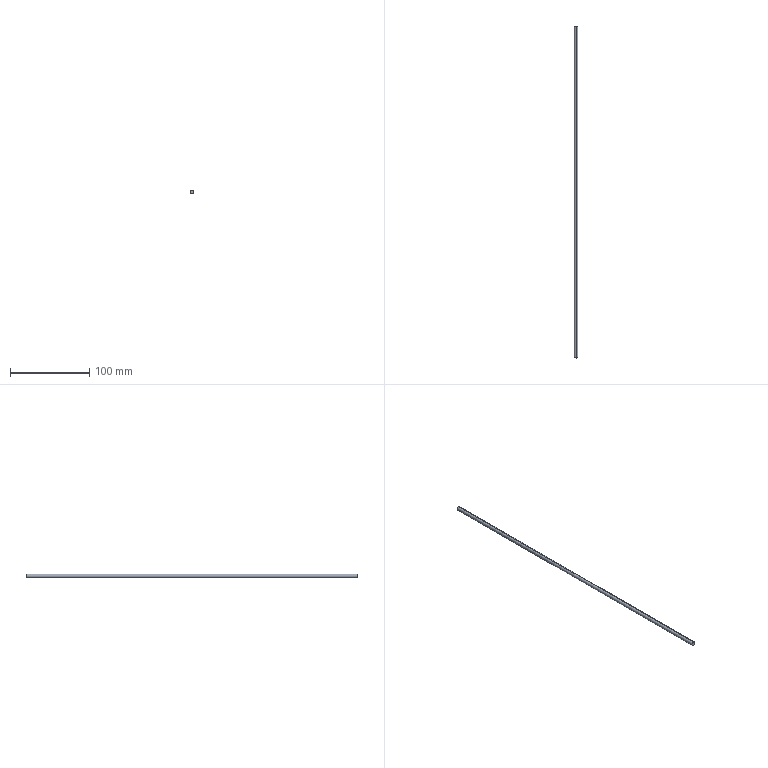Part | SolidWorks | features Extrusion 1 | 1 solid | 4 faces | box 5 x 420 x 5 mm | volume 8247 mm3 | cylinder 2 | plane 2 | commonest cylinder face diameters 5 x2
STEP:
#1=CARTESIAN_POINT('',(0.,420.,2.5));
#2=VERTEX_POINT('',#1);
#3=CARTESIAN_POINT('',(0.,420.,-2.5));
#4=VERTEX_POINT('',#3);
#5=CARTESIAN_POINT('',(0.,420.,0.));
#6=DIRECTION('',(0.,1.,0.));
#7=DIRECTION('',(0.,0.,1.));
#8=AXIS2_PLACEMENT_3D('',#5,#6,#7);
#9=CIRCLE('',#8,2.5);
#10=EDGE_CURVE('',#2,#4,#9,.T.);
#11=ORIENTED_EDGE('',*,*,#10,.F.);
#12=CARTESIAN_POINT('',(0.,0.,2.5));
#13=VERTEX_POINT('',#12);
#14=CARTESIAN_POINT('',(0.,420.,2.5));
#15=DIRECTION('',(0.,-1.,0.));
#16=VECTOR('',#15,1000.);
#17=LINE('',#14,#16);
#18=EDGE_CURVE('',#2,#13,#17,.T.);
#19=ORIENTED_EDGE('',*,*,#18,.T.);
#20=CARTESIAN_POINT('',(0.,0.,-2.5));
#21=VERTEX_POINT('',#20);
#22=CARTESIAN_POINT('',(0.,0.,0.));
#23=DIRECTION('',(0.,1.,0.));
#24=DIRECTION('',(0.,0.,1.));
#25=AXIS2_PLACEMENT_3D('',#22,#23,#24);
#26=CIRCLE('',#25,2.5);
#27=EDGE_CURVE('',#13,#21,#26,.T.);
#28=ORIENTED_EDGE('',*,*,#27,.T.);
#29=CARTESIAN_POINT('',(0.,420.,-2.5));
#30=DIRECTION('',(0.,-1.,0.));
#31=VECTOR('',#30,1000.);
#32=LINE('',#29,#31);
#33=EDGE_CURVE('',#4,#21,#32,.T.);
#34=ORIENTED_EDGE('',*,*,#33,.F.);
#35=EDGE_LOOP('',(#11,#19,#28,#34));
#36=FACE_OUTER_BOUND('',#35,.T.);
#37=CARTESIAN_POINT('',(0.,420.,0.));
#38=DIRECTION('',(0.,-1.,0.));
#39=DIRECTION('',(0.,0.,-1.));
#40=AXIS2_PLACEMENT_3D('',#37,#38,#39);
#41=CYLINDRICAL_SURFACE('',#40,2.5);
#42=ADVANCED_FACE('',(#36),#41,.T.);
#43=ORIENTED_EDGE('',*,*,#18,.F.);
#44=CARTESIAN_POINT('',(0.,420.,0.));
#45=DIRECTION('',(0.,1.,0.));
#46=DIRECTION('',(0.,0.,1.));
#47=AXIS2_PLACEMENT_3D('',#44,#45,#46);
#48=CIRCLE('',#47,2.5);
#49=EDGE_CURVE('',#4,#2,#48,.T.);
#50=ORIENTED_EDGE('',*,*,#49,.F.);
#51=ORIENTED_EDGE('',*,*,#33,.T.);
#52=CARTESIAN_POINT('',(0.,0.,0.));
#53=DIRECTION('',(0.,1.,0.));
#54=DIRECTION('',(0.,0.,1.));
#55=AXIS2_PLACEMENT_3D('',#52,#53,#54);
#56=CIRCLE('',#55,2.5);
#57=EDGE_CURVE('',#21,#13,#56,.T.);
#58=ORIENTED_EDGE('',*,*,#57,.T.);
#59=EDGE_LOOP('',(#43,#50,#51,#58));
#60=FACE_OUTER_BOUND('',#59,.T.);
#61=CARTESIAN_POINT('',(0.,420.,0.));
#62=DIRECTION('',(0.,-1.,0.));
#63=DIRECTION('',(0.,0.,-1.));
#64=AXIS2_PLACEMENT_3D('',#61,#62,#63);
#65=CYLINDRICAL_SURFACE('',#64,2.5);
#66=ADVANCED_FACE('',(#60),#65,.T.);
#67=ORIENTED_EDGE('',*,*,#49,.T.);
#68=ORIENTED_EDGE('',*,*,#10,.T.);
#69=EDGE_LOOP('',(#67,#68));
#70=FACE_OUTER_BOUND('',#69,.T.);
#71=CARTESIAN_POINT('',(0.,420.,0.));
#72=DIRECTION('',(0.,1.,0.));
#73=DIRECTION('',(0.,0.,1.));
#74=AXIS2_PLACEMENT_3D('',#71,#72,#73);
#75=PLANE('',#74);
#76=ADVANCED_FACE('',(#70),#75,.T.);
#77=ORIENTED_EDGE('',*,*,#57,.F.);
#78=ORIENTED_EDGE('',*,*,#27,.F.);
#79=EDGE_LOOP('',(#77,#78));
#80=FACE_OUTER_BOUND('',#79,.T.);
#81=CARTESIAN_POINT('',(0.,0.,0.));
#82=DIRECTION('',(0.,1.,0.));
#83=DIRECTION('',(0.,0.,1.));
#84=AXIS2_PLACEMENT_3D('',#81,#82,#83);
#85=PLANE('',#84);
#86=ADVANCED_FACE('',(#80),#85,.F.);
#87=CLOSED_SHELL('',(#42,#66,#76,#86));
#88=MANIFOLD_SOLID_BREP('',#87);
#89=CARTESIAN_POINT('',(0.,0.,0.));
#90=DIRECTION('',(0.,0.,1.));
#91=DIRECTION('',(1.,0.,0.));
#92=AXIS2_PLACEMENT_3D('',#89,#90,#91);
#93=(LENGTH_UNIT()NAMED_UNIT(*)SI_UNIT(.MILLI.,.METRE.));
#94=UNCERTAINTY_MEASURE_WITH_UNIT(LENGTH_MEASURE(0.00001),#93,'','');
#95=(NAMED_UNIT(*)PLANE_ANGLE_UNIT()SI_UNIT($,.RADIAN.));
#96=(NAMED_UNIT(*)SI_UNIT($,.STERADIAN.)SOLID_ANGLE_UNIT());
#97=(GEOMETRIC_REPRESENTATION_CONTEXT(3)GLOBAL_UNCERTAINTY_ASSIGNED_CONTEXT((#94))GLOBAL_UNIT_ASSIGNED_CONTEXT((#93,#95,#96))REPRESENTATION_CONTEXT('',''));
#98=ADVANCED_BREP_SHAPE_REPRESENTATION('',(#88,#92),#97);